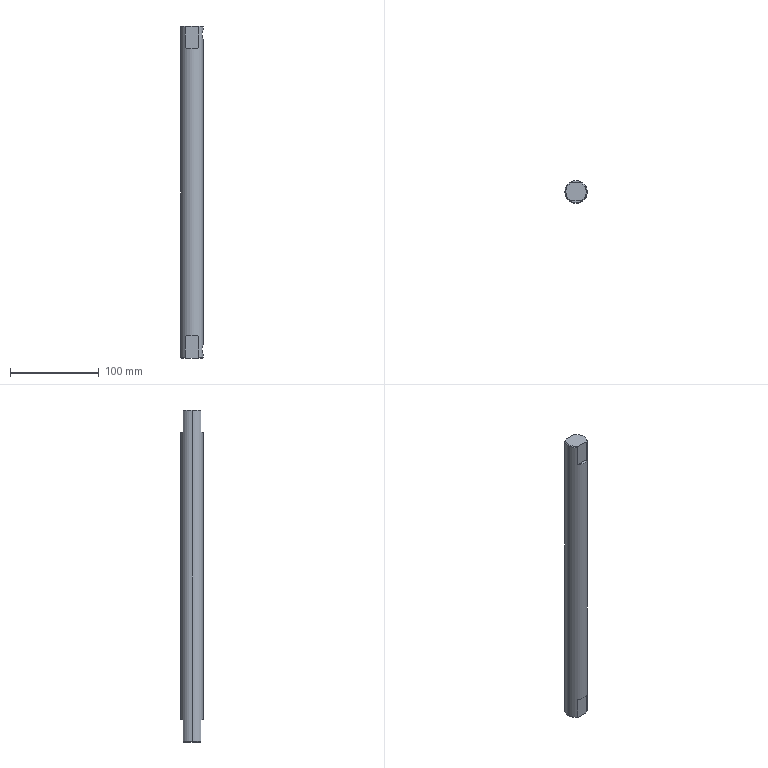Part | SolidWorks | features ICE 2, Chamfer 1, Extrusion 1, MirrorPattern 1 | 1 solid | 24 faces | box 25 x 25 x 374 mm | volume 180094 mm3 | plane 12 | cylinder 6 | cone 6 | commonest cylinder face diameters 11 x4 25 x2
STEP:
#1=CARTESIAN_POINT('',(7.5,0.,-172.));
#2=VERTEX_POINT('',#1);
#3=CARTESIAN_POINT('',(7.5,0.,-183.));
#4=VERTEX_POINT('',#3);
#5=CARTESIAN_POINT('',(7.5,0.,-177.5));
#6=DIRECTION('',(1.,0.,0.));
#7=DIRECTION('',(0.,0.,1.));
#8=AXIS2_PLACEMENT_3D('',#5,#6,#7);
#9=CIRCLE('',#8,5.5);
#10=EDGE_CURVE('',#2,#4,#9,.T.);
#11=ORIENTED_EDGE('',*,*,#10,.F.);
#12=CARTESIAN_POINT('',(12.5,0.,-172.));
#13=VERTEX_POINT('',#12);
#14=CARTESIAN_POINT('',(7.5,0.,-172.));
#15=DIRECTION('',(1.,0.,0.));
#16=VECTOR('',#15,1000.);
#17=LINE('',#14,#16);
#18=EDGE_CURVE('',#2,#13,#17,.T.);
#19=ORIENTED_EDGE('',*,*,#18,.T.);
#20=CARTESIAN_POINT('',(12.5,0.,-183.));
#21=VERTEX_POINT('',#20);
#22=CARTESIAN_POINT('',(12.5,0.,-183.));
#23=CARTESIAN_POINT('',(12.5,-0.3685,-183.));
#24=CARTESIAN_POINT('',(12.484,-0.73,-182.963));
#25=CARTESIAN_POINT('',(12.422,-1.44,-182.821));
#26=CARTESIAN_POINT('',(12.376,-1.792,-182.712));
#27=CARTESIAN_POINT('',(12.261,-2.456,-182.434));
#28=CARTESIAN_POINT('',(12.193,-2.77,-182.265));
#29=CARTESIAN_POINT('',(12.08,-3.216,-181.965));
#30=CARTESIAN_POINT('',(12.041,-3.361,-181.857));
#31=CARTESIAN_POINT('',(11.96,-3.636,-181.631));
#32=CARTESIAN_POINT('',(11.92,-3.767,-181.511));
#33=CARTESIAN_POINT('',(11.797,-4.142,-181.135));
#34=CARTESIAN_POINT('',(11.713,-4.369,-180.86));
#35=CARTESIAN_POINT('',(11.557,-4.768,-180.264));
#36=CARTESIAN_POINT('',(11.485,-4.937,-179.951));
#37=CARTESIAN_POINT('',(11.393,-5.144,-179.456));
#38=CARTESIAN_POINT('',(11.365,-5.205,-179.287));
#39=CARTESIAN_POINT('',(11.316,-5.311,-178.94));
#40=CARTESIAN_POINT('',(11.294,-5.356,-178.762));
#41=CARTESIAN_POINT('',(11.243,-5.464,-178.228));
#42=CARTESIAN_POINT('',(11.225,-5.5,-177.868));
#43=CARTESIAN_POINT('',(11.225,-5.5,-177.322));
#44=CARTESIAN_POINT('',(11.229,-5.491,-177.138));
#45=CARTESIAN_POINT('',(11.247,-5.455,-176.773));
#46=CARTESIAN_POINT('',(11.26,-5.428,-176.593));
#47=CARTESIAN_POINT('',(11.311,-5.321,-176.06));
#48=CARTESIAN_POINT('',(11.362,-5.214,-175.713));
#49=CARTESIAN_POINT('',(11.486,-4.935,-175.045));
#50=CARTESIAN_POINT('',(11.558,-4.765,-174.731));
#51=CARTESIAN_POINT('',(11.714,-4.369,-174.14));
#52=CARTESIAN_POINT('',(11.798,-4.139,-173.861));
#53=CARTESIAN_POINT('',(11.962,-3.637,-173.359));
#54=CARTESIAN_POINT('',(12.043,-3.364,-173.134));
#55=CARTESIAN_POINT('',(12.156,-2.918,-172.834));
#56=CARTESIAN_POINT('',(12.192,-2.763,-172.741));
#57=CARTESIAN_POINT('',(12.259,-2.446,-172.571));
#58=CARTESIAN_POINT('',(12.291,-2.285,-172.494));
#59=CARTESIAN_POINT('',(12.376,-1.789,-172.287));
#60=CARTESIAN_POINT('',(12.422,-1.445,-172.18));
#61=CARTESIAN_POINT('',(12.484,-0.7246,-172.036));
#62=CARTESIAN_POINT('',(12.5,-0.3631,-172.));
#63=CARTESIAN_POINT('',(12.5,0.,-172.));
#64=B_SPLINE_CURVE_WITH_KNOTS('',3,(#22,#23,#24,#25,#26,#27,#28,#29,#30,#31,#32,#33,#34,#35,#36,#37,#38,#39,#40,#41,#42,#43,#44,#45,#46,#47,#48,#49,#50,#51,#52,#53,#54,#55,#56,#57,#58,#59,#60,#61,#62,#63),.UNSPECIFIED.,.F.,.F.,(4,2,2,2,2,2,2,2,2,2,2,2,2,2,2,2,2,2,2,2,4),(0.,0.001089,0.002178,0.003267,0.003811,0.004355,0.005444,0.006533,0.007078,0.007622,0.008711,0.009255,0.0098,0.01089,0.01198,0.01307,0.01416,0.0147,0.01524,0.01633,0.01742),.UNSPECIFIED.);
#65=EDGE_CURVE('',#21,#13,#64,.T.);
#66=ORIENTED_EDGE('',*,*,#65,.F.);
#67=CARTESIAN_POINT('',(7.5,0.,-183.));
#68=DIRECTION('',(1.,0.,0.));
#69=VECTOR('',#68,1000.);
#70=LINE('',#67,#69);
#71=EDGE_CURVE('',#4,#21,#70,.T.);
#72=ORIENTED_EDGE('',*,*,#71,.F.);
#73=EDGE_LOOP('',(#11,#19,#66,#72));
#74=FACE_OUTER_BOUND('',#73,.T.);
#75=CARTESIAN_POINT('',(7.5,0.,-177.5));
#76=DIRECTION('',(1.,0.,0.));
#77=DIRECTION('',(0.,0.,-1.));
#78=AXIS2_PLACEMENT_3D('',#75,#76,#77);
#79=CYLINDRICAL_SURFACE('',#78,5.5);
#80=ADVANCED_FACE('',(#74),#79,.F.);
#81=CARTESIAN_POINT('',(7.5,0.,183.));
#82=VERTEX_POINT('',#81);
#83=CARTESIAN_POINT('',(7.5,0.,172.));
#84=VERTEX_POINT('',#83);
#85=CARTESIAN_POINT('',(7.5,0.,177.5));
#86=DIRECTION('',(1.,0.,0.));
#87=DIRECTION('',(0.,0.,-1.));
#88=AXIS2_PLACEMENT_3D('',#85,#86,#87);
#89=CIRCLE('',#88,5.5);
#90=EDGE_CURVE('',#82,#84,#89,.T.);
#91=ORIENTED_EDGE('',*,*,#90,.F.);
#92=CARTESIAN_POINT('',(12.5,0.,183.));
#93=VERTEX_POINT('',#92);
#94=CARTESIAN_POINT('',(7.5,0.,183.));
#95=DIRECTION('',(1.,0.,0.));
#96=VECTOR('',#95,1000.);
#97=LINE('',#94,#96);
#98=EDGE_CURVE('',#82,#93,#97,.T.);
#99=ORIENTED_EDGE('',*,*,#98,.T.);
#100=CARTESIAN_POINT('',(12.5,0.,172.));
#101=VERTEX_POINT('',#100);
#102=CARTESIAN_POINT('',(12.5,0.,172.));
#103=CARTESIAN_POINT('',(12.5,-0.3685,172.));
#104=CARTESIAN_POINT('',(12.484,-0.73,172.037));
#105=CARTESIAN_POINT('',(12.422,-1.44,172.179));
#106=CARTESIAN_POINT('',(12.376,-1.792,172.288));
#107=CARTESIAN_POINT('',(12.261,-2.456,172.566));
#108=CARTESIAN_POINT('',(12.193,-2.77,172.735));
#109=CARTESIAN_POINT('',(12.08,-3.216,173.035));
#110=CARTESIAN_POINT('',(12.041,-3.361,173.143));
#111=CARTESIAN_POINT('',(11.96,-3.636,173.369));
#112=CARTESIAN_POINT('',(11.92,-3.767,173.489));
#113=CARTESIAN_POINT('',(11.797,-4.142,173.865));
#114=CARTESIAN_POINT('',(11.713,-4.369,174.14));
#115=CARTESIAN_POINT('',(11.557,-4.768,174.736));
#116=CARTESIAN_POINT('',(11.485,-4.937,175.049));
#117=CARTESIAN_POINT('',(11.393,-5.144,175.544));
#118=CARTESIAN_POINT('',(11.365,-5.205,175.713));
#119=CARTESIAN_POINT('',(11.316,-5.311,176.06));
#120=CARTESIAN_POINT('',(11.294,-5.356,176.238));
#121=CARTESIAN_POINT('',(11.243,-5.464,176.772));
#122=CARTESIAN_POINT('',(11.225,-5.5,177.132));
#123=CARTESIAN_POINT('',(11.225,-5.5,177.678));
#124=CARTESIAN_POINT('',(11.229,-5.491,177.862));
#125=CARTESIAN_POINT('',(11.247,-5.455,178.227));
#126=CARTESIAN_POINT('',(11.26,-5.428,178.407));
#127=CARTESIAN_POINT('',(11.311,-5.321,178.94));
#128=CARTESIAN_POINT('',(11.362,-5.214,179.287));
#129=CARTESIAN_POINT('',(11.486,-4.935,179.955));
#130=CARTESIAN_POINT('',(11.558,-4.765,180.269));
#131=CARTESIAN_POINT('',(11.714,-4.369,180.86));
#132=CARTESIAN_POINT('',(11.798,-4.139,181.139));
#133=CARTESIAN_POINT('',(11.962,-3.637,181.641));
#134=CARTESIAN_POINT('',(12.043,-3.364,181.866));
#135=CARTESIAN_POINT('',(12.156,-2.918,182.166));
#136=CARTESIAN_POINT('',(12.192,-2.763,182.259));
#137=CARTESIAN_POINT('',(12.259,-2.446,182.429));
#138=CARTESIAN_POINT('',(12.291,-2.285,182.506));
#139=CARTESIAN_POINT('',(12.376,-1.789,182.713));
#140=CARTESIAN_POINT('',(12.422,-1.445,182.82));
#141=CARTESIAN_POINT('',(12.484,-0.7246,182.964));
#142=CARTESIAN_POINT('',(12.5,-0.3631,183.));
#143=CARTESIAN_POINT('',(12.5,0.,183.));
#144=B_SPLINE_CURVE_WITH_KNOTS('',3,(#102,#103,#104,#105,#106,#107,#108,#109,#110,#111,#112,#113,#114,#115,#116,#117,#118,#119,#120,#121,#122,#123,#124,#125,#126,#127,#128,#129,#130,#131,#132,#133,#134,#135,#136,#137,#138,#139,#140,#141,#142,#143),.UNSPECIFIED.,.F.,.F.,(4,2,2,2,2,2,2,2,2,2,2,2,2,2,2,2,2,2,2,2,4),(0.,0.001089,0.002178,0.003267,0.003811,0.004355,0.005444,0.006533,0.007078,0.007622,0.008711,0.009255,0.0098,0.01089,0.01198,0.01307,0.01416,0.0147,0.01524,0.01633,0.01742),.UNSPECIFIED.);
#145=EDGE_CURVE('',#101,#93,#144,.T.);
#146=ORIENTED_EDGE('',*,*,#145,.F.);
#147=CARTESIAN_POINT('',(7.5,0.,172.));
#148=DIRECTION('',(1.,0.,0.));
#149=VECTOR('',#148,1000.);
#150=LINE('',#147,#149);
#151=EDGE_CURVE('',#84,#101,#150,.T.);
#152=ORIENTED_EDGE('',*,*,#151,.F.);
#153=EDGE_LOOP('',(#91,#99,#146,#152));
#154=FACE_OUTER_BOUND('',#153,.T.);
#155=CARTESIAN_POINT('',(7.5,0.,177.5));
#156=DIRECTION('',(1.,0.,0.));
#157=DIRECTION('',(0.,0.,-1.));
#158=AXIS2_PLACEMENT_3D('',#155,#156,#157);
#159=CYLINDRICAL_SURFACE('',#158,5.5);
#160=ADVANCED_FACE('',(#154),#159,.F.);
#161=CARTESIAN_POINT('',(-11.5,0.,187.));
#162=VERTEX_POINT('',#161);
#163=CARTESIAN_POINT('',(-5.679,-10.,187.));
#164=VERTEX_POINT('',#163);
#165=CARTESIAN_POINT('',(0.,0.,187.));
#166=DIRECTION('',(0.,0.,1.));
#167=DIRECTION('',(1.,0.,0.));
#168=AXIS2_PLACEMENT_3D('',#165,#166,#167);
#169=CIRCLE('',#168,11.5);
#170=EDGE_CURVE('',#162,#164,#169,.T.);
#171=ORIENTED_EDGE('',*,*,#170,.F.);
#172=CARTESIAN_POINT('',(-12.5,0.,186.));
#173=VERTEX_POINT('',#172);
#174=CARTESIAN_POINT('',(-11.5,0.,187.));
#175=DIRECTION('',(-0.7071,0.,-0.7071));
#176=VECTOR('',#175,1000.);
#177=LINE('',#174,#176);
#178=EDGE_CURVE('',#162,#173,#177,.T.);
#179=ORIENTED_EDGE('',*,*,#178,.T.);
#180=CARTESIAN_POINT('',(-7.5,-10.,186.));
#181=VERTEX_POINT('',#180);
#182=CARTESIAN_POINT('',(0.,0.,186.));
#183=DIRECTION('',(0.,0.,-1.));
#184=DIRECTION('',(1.,0.,0.));
#185=AXIS2_PLACEMENT_3D('',#182,#183,#184);
#186=CIRCLE('',#185,12.5);
#187=EDGE_CURVE('',#181,#173,#186,.T.);
#188=ORIENTED_EDGE('',*,*,#187,.F.);
#189=CARTESIAN_POINT('',(-5.679,-10.,187.));
#190=CARTESIAN_POINT('',(-6.301,-10.,186.693));
#191=CARTESIAN_POINT('',(-6.906,-10.,186.356));
#192=CARTESIAN_POINT('',(-7.5,-10.,186.));
#193=B_SPLINE_CURVE_WITH_KNOTS('',3,(#189,#190,#191,#192),.UNSPECIFIED.,.F.,.F.,(4,4),(0.03752,0.03962),.UNSPECIFIED.);
#194=EDGE_CURVE('',#164,#181,#193,.T.);
#195=ORIENTED_EDGE('',*,*,#194,.F.);
#196=EDGE_LOOP('',(#171,#179,#188,#195));
#197=FACE_OUTER_BOUND('',#196,.T.);
#198=CARTESIAN_POINT('',(0.,0.,187.));
#199=DIRECTION('',(0.,0.,-1.));
#200=DIRECTION('',(-1.,0.,0.));
#201=AXIS2_PLACEMENT_3D('',#198,#199,#200);
#202=CONICAL_SURFACE('',#201,11.5,0.7854);
#203=ADVANCED_FACE('',(#197),#202,.T.);
#204=CARTESIAN_POINT('',(11.5,0.,-187.));
#205=VERTEX_POINT('',#204);
#206=CARTESIAN_POINT('',(5.679,-10.,-187.));
#207=VERTEX_POINT('',#206);
#208=CARTESIAN_POINT('',(0.,0.,-187.));
#209=DIRECTION('',(0.,0.,-1.));
#210=DIRECTION('',(1.,0.,0.));
#211=AXIS2_PLACEMENT_3D('',#208,#209,#210);
#212=CIRCLE('',#211,11.5);
#213=EDGE_CURVE('',#205,#207,#212,.T.);
#214=ORIENTED_EDGE('',*,*,#213,.F.);
#215=CARTESIAN_POINT('',(12.5,0.,-186.));
#216=VERTEX_POINT('',#215);
#217=CARTESIAN_POINT('',(12.5,0.,-186.));
#218=DIRECTION('',(0.7071,0.,0.7071));
#219=VECTOR('',#218,1000.);
#220=LINE('',#217,#219);
#221=EDGE_CURVE('',#205,#216,#220,.T.);
#222=ORIENTED_EDGE('',*,*,#221,.T.);
#223=CARTESIAN_POINT('',(7.5,-10.,-186.));
#224=VERTEX_POINT('',#223);
#225=CARTESIAN_POINT('',(0.,0.,-186.));
#226=DIRECTION('',(0.,0.,1.));
#227=DIRECTION('',(1.,0.,0.));
#228=AXIS2_PLACEMENT_3D('',#225,#226,#227);
#229=CIRCLE('',#228,12.5);
#230=EDGE_CURVE('',#224,#216,#229,.T.);
#231=ORIENTED_EDGE('',*,*,#230,.F.);
#232=CARTESIAN_POINT('',(7.5,-10.,-186.));
#233=CARTESIAN_POINT('',(6.905,-10.,-186.357));
#234=CARTESIAN_POINT('',(6.299,-10.,-186.694));
#235=CARTESIAN_POINT('',(5.679,-10.,-187.));
#236=B_SPLINE_CURVE_WITH_KNOTS('',3,(#232,#233,#234,#235),.UNSPECIFIED.,.F.,.F.,(4,4),(0.02358,0.02565),.UNSPECIFIED.);
#237=EDGE_CURVE('',#224,#207,#236,.T.);
#238=ORIENTED_EDGE('',*,*,#237,.T.);
#239=EDGE_LOOP('',(#214,#222,#231,#238));
#240=FACE_OUTER_BOUND('',#239,.T.);
#241=CARTESIAN_POINT('',(0.,0.,-186.));
#242=DIRECTION('',(0.,0.,1.));
#243=DIRECTION('',(1.,0.,0.));
#244=AXIS2_PLACEMENT_3D('',#241,#242,#243);
#245=CONICAL_SURFACE('',#244,12.5,0.7854);
#246=ADVANCED_FACE('',(#240),#245,.T.);
#247=CARTESIAN_POINT('',(7.5,10.,186.));
#248=VERTEX_POINT('',#247);
#249=CARTESIAN_POINT('',(12.5,0.,186.));
#250=VERTEX_POINT('',#249);
#251=CARTESIAN_POINT('',(0.,0.,186.));
#252=DIRECTION('',(0.,0.,-1.));
#253=DIRECTION('',(1.,0.,0.));
#254=AXIS2_PLACEMENT_3D('',#251,#252,#253);
#255=CIRCLE('',#254,12.5);
#256=EDGE_CURVE('',#248,#250,#255,.T.);
#257=ORIENTED_EDGE('',*,*,#256,.T.);
#258=CARTESIAN_POINT('',(12.5,0.,187.));
#259=DIRECTION('',(0.,0.,-1.));
#260=VECTOR('',#259,1000.);
#261=LINE('',#258,#260);
#262=EDGE_CURVE('',#250,#93,#261,.T.);
#263=ORIENTED_EDGE('',*,*,#262,.T.);
#264=CARTESIAN_POINT('',(12.5,0.,183.));
#265=CARTESIAN_POINT('',(12.5,0.1813,183.));
#266=CARTESIAN_POINT('',(12.496,0.3631,182.991));
#267=CARTESIAN_POINT('',(12.48,0.7273,182.955));
#268=CARTESIAN_POINT('',(12.468,0.9095,182.927));
#269=CARTESIAN_POINT('',(12.421,1.444,182.82));
#270=CARTESIAN_POINT('',(12.376,1.788,182.714));
#271=CARTESIAN_POINT('',(12.29,2.289,182.505));
#272=CARTESIAN_POINT('',(12.258,2.453,182.426));
#273=CARTESIAN_POINT('',(12.191,2.769,182.256));
#274=CARTESIAN_POINT('',(12.155,2.921,182.163));
#275=CARTESIAN_POINT('',(12.043,3.364,181.866));
#276=CARTESIAN_POINT('',(11.961,3.641,181.637));
#277=CARTESIAN_POINT('',(11.796,4.145,181.133));
#278=CARTESIAN_POINT('',(11.713,4.369,180.859));
#279=CARTESIAN_POINT('',(11.558,4.765,180.27));
#280=CARTESIAN_POINT('',(11.484,4.938,179.949));
#281=CARTESIAN_POINT('',(11.362,5.214,179.288));
#282=CARTESIAN_POINT('',(11.312,5.319,178.945));
#283=CARTESIAN_POINT('',(11.261,5.427,178.412));
#284=CARTESIAN_POINT('',(11.247,5.454,178.229));
#285=CARTESIAN_POINT('',(11.229,5.491,177.866));
#286=CARTESIAN_POINT('',(11.225,5.5,177.684));
#287=CARTESIAN_POINT('',(11.225,5.5,177.14));
#288=CARTESIAN_POINT('',(11.243,5.465,176.777));
#289=CARTESIAN_POINT('',(11.311,5.32,176.059));
#290=CARTESIAN_POINT('',(11.361,5.214,175.714));
#291=CARTESIAN_POINT('',(11.484,4.938,175.051));
#292=CARTESIAN_POINT('',(11.558,4.766,174.731));
#293=CARTESIAN_POINT('',(11.713,4.369,174.14));
#294=CARTESIAN_POINT('',(11.796,4.144,173.866));
#295=CARTESIAN_POINT('',(11.962,3.639,173.36));
#296=CARTESIAN_POINT('',(12.043,3.363,173.134));
#297=CARTESIAN_POINT('',(12.155,2.921,172.837));
#298=CARTESIAN_POINT('',(12.191,2.769,172.744));
#299=CARTESIAN_POINT('',(12.258,2.454,172.574));
#300=CARTESIAN_POINT('',(12.29,2.29,172.496));
#301=CARTESIAN_POINT('',(12.376,1.789,172.286));
#302=CARTESIAN_POINT('',(12.421,1.445,172.181));
#303=CARTESIAN_POINT('',(12.483,0.7361,172.038));
#304=CARTESIAN_POINT('',(12.5,0.3681,172.));
#305=CARTESIAN_POINT('',(12.5,0.,172.));
#306=B_SPLINE_CURVE_WITH_KNOTS('',3,(#264,#265,#266,#267,#268,#269,#270,#271,#272,#273,#274,#275,#276,#277,#278,#279,#280,#281,#282,#283,#284,#285,#286,#287,#288,#289,#290,#291,#292,#293,#294,#295,#296,#297,#298,#299,#300,#301,#302,#303,#304,#305),.UNSPECIFIED.,.F.,.F.,(4,2,2,2,2,2,2,2,2,2,2,2,2,2,2,2,2,2,2,2,4),(0.01742,0.01797,0.01851,0.0196,0.02014,0.02068,0.02177,0.02286,0.02395,0.02504,0.02558,0.02612,0.02721,0.0283,0.02939,0.03047,0.03156,0.03211,0.03265,0.03374,0.03483),.UNSPECIFIED.);
#307=EDGE_CURVE('',#93,#101,#306,.T.);
#308=ORIENTED_EDGE('',*,*,#307,.T.);
#309=CARTESIAN_POINT('',(12.5,0.,187.));
#310=DIRECTION('',(0.,0.,-1.));
#311=VECTOR('',#310,1000.);
#312=LINE('',#309,#311);
#313=EDGE_CURVE('',#101,#13,#312,.T.);
#314=ORIENTED_EDGE('',*,*,#313,.T.);
#315=CARTESIAN_POINT('',(12.5,0.,-172.));
#316=CARTESIAN_POINT('',(12.5,0.1813,-172.));
#317=CARTESIAN_POINT('',(12.496,0.3631,-172.009));
#318=CARTESIAN_POINT('',(12.48,0.7273,-172.045));
#319=CARTESIAN_POINT('',(12.468,0.9095,-172.073));
#320=CARTESIAN_POINT('',(12.421,1.444,-172.18));
#321=CARTESIAN_POINT('',(12.376,1.788,-172.286));
#322=CARTESIAN_POINT('',(12.29,2.289,-172.495));
#323=CARTESIAN_POINT('',(12.258,2.453,-172.574));
#324=CARTESIAN_POINT('',(12.191,2.769,-172.744));
#325=CARTESIAN_POINT('',(12.155,2.921,-172.837));
#326=CARTESIAN_POINT('',(12.043,3.364,-173.134));
#327=CARTESIAN_POINT('',(11.961,3.641,-173.363));
#328=CARTESIAN_POINT('',(11.796,4.145,-173.867));
#329=CARTESIAN_POINT('',(11.713,4.369,-174.141));
#330=CARTESIAN_POINT('',(11.558,4.765,-174.73));
#331=CARTESIAN_POINT('',(11.484,4.938,-175.051));
#332=CARTESIAN_POINT('',(11.362,5.214,-175.712));
#333=CARTESIAN_POINT('',(11.312,5.319,-176.055));
#334=CARTESIAN_POINT('',(11.261,5.427,-176.588));
#335=CARTESIAN_POINT('',(11.247,5.454,-176.771));
#336=CARTESIAN_POINT('',(11.229,5.491,-177.134));
#337=CARTESIAN_POINT('',(11.225,5.5,-177.316));
#338=CARTESIAN_POINT('',(11.225,5.5,-177.86));
#339=CARTESIAN_POINT('',(11.243,5.465,-178.223));
#340=CARTESIAN_POINT('',(11.311,5.32,-178.941));
#341=CARTESIAN_POINT('',(11.361,5.214,-179.286));
#342=CARTESIAN_POINT('',(11.484,4.938,-179.949));
#343=CARTESIAN_POINT('',(11.558,4.766,-180.269));
#344=CARTESIAN_POINT('',(11.713,4.369,-180.86));
#345=CARTESIAN_POINT('',(11.796,4.144,-181.134));
#346=CARTESIAN_POINT('',(11.962,3.639,-181.64));
#347=CARTESIAN_POINT('',(12.043,3.363,-181.866));
#348=CARTESIAN_POINT('',(12.155,2.921,-182.163));
#349=CARTESIAN_POINT('',(12.191,2.769,-182.256));
#350=CARTESIAN_POINT('',(12.258,2.454,-182.426));
#351=CARTESIAN_POINT('',(12.29,2.29,-182.504));
#352=CARTESIAN_POINT('',(12.376,1.789,-182.714));
#353=CARTESIAN_POINT('',(12.421,1.445,-182.819));
#354=CARTESIAN_POINT('',(12.483,0.7361,-182.962));
#355=CARTESIAN_POINT('',(12.5,0.3681,-183.));
#356=CARTESIAN_POINT('',(12.5,0.,-183.));
#357=B_SPLINE_CURVE_WITH_KNOTS('',3,(#315,#316,#317,#318,#319,#320,#321,#322,#323,#324,#325,#326,#327,#328,#329,#330,#331,#332,#333,#334,#335,#336,#337,#338,#339,#340,#341,#342,#343,#344,#345,#346,#347,#348,#349,#350,#351,#352,#353,#354,#355,#356),.UNSPECIFIED.,.F.,.F.,(4,2,2,2,2,2,2,2,2,2,2,2,2,2,2,2,2,2,2,2,4),(0.01742,0.01797,0.01851,0.0196,0.02014,0.02068,0.02177,0.02286,0.02395,0.02504,0.02558,0.02612,0.02721,0.0283,0.02939,0.03047,0.03156,0.03211,0.03265,0.03374,0.03483),.UNSPECIFIED.);
#358=EDGE_CURVE('',#13,#21,#357,.T.);
#359=ORIENTED_EDGE('',*,*,#358,.T.);
#360=CARTESIAN_POINT('',(12.5,0.,187.));
#361=DIRECTION('',(0.,0.,-1.));
#362=VECTOR('',#361,1000.);
#363=LINE('',#360,#362);
#364=EDGE_CURVE('',#21,#216,#363,.T.);
#365=ORIENTED_EDGE('',*,*,#364,.T.);
#366=CARTESIAN_POINT('',(7.5,10.,-186.));
#367=VERTEX_POINT('',#366);
#368=CARTESIAN_POINT('',(0.,0.,-186.));
#369=DIRECTION('',(0.,0.,1.));
#370=DIRECTION('',(1.,0.,0.));
#371=AXIS2_PLACEMENT_3D('',#368,#369,#370);
#372=CIRCLE('',#371,12.5);
#373=EDGE_CURVE('',#216,#367,#372,.T.);
#374=ORIENTED_EDGE('',*,*,#373,.T.);
#375=CARTESIAN_POINT('',(7.5,10.,-162.));
#376=VERTEX_POINT('',#375);
#377=CARTESIAN_POINT('',(7.5,10.,187.));
#378=DIRECTION('',(0.,0.,-1.));
#379=VECTOR('',#378,1000.);
#380=LINE('',#377,#379);
#381=EDGE_CURVE('',#376,#367,#380,.T.);
#382=ORIENTED_EDGE('',*,*,#381,.F.);
#383=CARTESIAN_POINT('',(-7.5,10.,-162.));
#384=VERTEX_POINT('',#383);
#385=CARTESIAN_POINT('',(0.,0.,-162.));
#386=DIRECTION('',(0.,0.,1.));
#387=DIRECTION('',(1.,0.,0.));
#388=AXIS2_PLACEMENT_3D('',#385,#386,#387);
#389=CIRCLE('',#388,12.5);
#390=EDGE_CURVE('',#376,#384,#389,.T.);
#391=ORIENTED_EDGE('',*,*,#390,.T.);
#392=CARTESIAN_POINT('',(-7.5,10.,-186.));
#393=VERTEX_POINT('',#392);
#394=CARTESIAN_POINT('',(-7.5,10.,187.));
#395=DIRECTION('',(0.,0.,1.));
#396=VECTOR('',#395,1000.);
#397=LINE('',#394,#396);
#398=EDGE_CURVE('',#393,#384,#397,.T.);
#399=ORIENTED_EDGE('',*,*,#398,.F.);
#400=CARTESIAN_POINT('',(-12.5,0.,-186.));
#401=VERTEX_POINT('',#400);
#402=CARTESIAN_POINT('',(0.,0.,-186.));
#403=DIRECTION('',(0.,0.,1.));
#404=DIRECTION('',(1.,0.,0.));
#405=AXIS2_PLACEMENT_3D('',#402,#403,#404);
#406=CIRCLE('',#405,12.5);
#407=EDGE_CURVE('',#393,#401,#406,.T.);
#408=ORIENTED_EDGE('',*,*,#407,.T.);
#409=CARTESIAN_POINT('',(-12.5,0.,187.));
#410=DIRECTION('',(0.,0.,-1.));
#411=VECTOR('',#410,1000.);
#412=LINE('',#409,#411);
#413=EDGE_CURVE('',#173,#401,#412,.T.);
#414=ORIENTED_EDGE('',*,*,#413,.F.);
#415=CARTESIAN_POINT('',(-7.5,10.,186.));
#416=VERTEX_POINT('',#415);
#417=CARTESIAN_POINT('',(0.,0.,186.));
#418=DIRECTION('',(0.,0.,-1.));
#419=DIRECTION('',(1.,0.,0.));
#420=AXIS2_PLACEMENT_3D('',#417,#418,#419);
#421=CIRCLE('',#420,12.5);
#422=EDGE_CURVE('',#173,#416,#421,.T.);
#423=ORIENTED_EDGE('',*,*,#422,.T.);
#424=CARTESIAN_POINT('',(-7.5,10.,162.));
#425=VERTEX_POINT('',#424);
#426=CARTESIAN_POINT('',(-7.5,10.,187.));
#427=DIRECTION('',(0.,0.,-1.));
#428=VECTOR('',#427,1000.);
#429=LINE('',#426,#428);
#430=EDGE_CURVE('',#416,#425,#429,.T.);
#431=ORIENTED_EDGE('',*,*,#430,.T.);
#432=CARTESIAN_POINT('',(7.5,10.,162.));
#433=VERTEX_POINT('',#432);
#434=CARTESIAN_POINT('',(0.,0.,162.));
#435=DIRECTION('',(0.,0.,-1.));
#436=DIRECTION('',(-1.,0.,0.));
#437=AXIS2_PLACEMENT_3D('',#434,#435,#436);
#438=CIRCLE('',#437,12.5);
#439=EDGE_CURVE('',#425,#433,#438,.T.);
#440=ORIENTED_EDGE('',*,*,#439,.T.);
#441=CARTESIAN_POINT('',(7.5,10.,187.));
#442=DIRECTION('',(0.,0.,1.));
#443=VECTOR('',#442,1000.);
#444=LINE('',#441,#443);
#445=EDGE_CURVE('',#433,#248,#444,.T.);
#446=ORIENTED_EDGE('',*,*,#445,.T.);
#447=EDGE_LOOP('',(#257,#263,#308,#314,#359,#365,#374,#382,#391,#399,#408,#414,#423,#431,#440,#446));
#448=FACE_OUTER_BOUND('',#447,.T.);
#449=CARTESIAN_POINT('',(0.,0.,187.));
#450=DIRECTION('',(0.,0.,-1.));
#451=DIRECTION('',(-1.,0.,0.));
#452=AXIS2_PLACEMENT_3D('',#449,#450,#451);
#453=CYLINDRICAL_SURFACE('',#452,12.5);
#454=ADVANCED_FACE('',(#448),#453,.T.);
#455=ORIENTED_EDGE('',*,*,#262,.F.);
#456=CARTESIAN_POINT('',(7.5,-10.,186.));
#457=VERTEX_POINT('',#456);
#458=CARTESIAN_POINT('',(0.,0.,186.));
#459=DIRECTION('',(0.,0.,-1.));
#460=DIRECTION('',(1.,0.,0.));
#461=AXIS2_PLACEMENT_3D('',#458,#459,#460);
#462=CIRCLE('',#461,12.5);
#463=EDGE_CURVE('',#250,#457,#462,.T.);
#464=ORIENTED_EDGE('',*,*,#463,.T.);
#465=CARTESIAN_POINT('',(7.5,-10.,162.));
#466=VERTEX_POINT('',#465);
#467=CARTESIAN_POINT('',(7.5,-10.,187.));
#468=DIRECTION('',(0.,0.,-1.));
#469=VECTOR('',#468,1000.);
#470=LINE('',#467,#469);
#471=EDGE_CURVE('',#457,#466,#470,.T.);
#472=ORIENTED_EDGE('',*,*,#471,.T.);
#473=CARTESIAN_POINT('',(-7.5,-10.,162.));
#474=VERTEX_POINT('',#473);
#475=CARTESIAN_POINT('',(0.,0.,162.));
#476=DIRECTION('',(0.,0.,1.));
#477=DIRECTION('',(1.,0.,0.));
#478=AXIS2_PLACEMENT_3D('',#475,#476,#477);
#479=CIRCLE('',#478,12.5);
#480=EDGE_CURVE('',#474,#466,#479,.T.);
#481=ORIENTED_EDGE('',*,*,#480,.F.);
#482=CARTESIAN_POINT('',(-7.5,-10.,187.));
#483=DIRECTION('',(0.,0.,1.));
#484=VECTOR('',#483,1000.);
#485=LINE('',#482,#484);
#486=EDGE_CURVE('',#474,#181,#485,.T.);
#487=ORIENTED_EDGE('',*,*,#486,.T.);
#488=ORIENTED_EDGE('',*,*,#187,.T.);
#489=ORIENTED_EDGE('',*,*,#413,.T.);
#490=CARTESIAN_POINT('',(-7.5,-10.,-186.));
#491=VERTEX_POINT('',#490);
#492=CARTESIAN_POINT('',(0.,0.,-186.));
#493=DIRECTION('',(0.,0.,1.));
#494=DIRECTION('',(1.,0.,0.));
#495=AXIS2_PLACEMENT_3D('',#492,#493,#494);
#496=CIRCLE('',#495,12.5);
#497=EDGE_CURVE('',#401,#491,#496,.T.);
#498=ORIENTED_EDGE('',*,*,#497,.T.);
#499=CARTESIAN_POINT('',(-7.5,-10.,-162.));
#500=VERTEX_POINT('',#499);
#501=CARTESIAN_POINT('',(-7.5,-10.,187.));
#502=DIRECTION('',(0.,0.,-1.));
#503=VECTOR('',#502,1000.);
#504=LINE('',#501,#503);
#505=EDGE_CURVE('',#500,#491,#504,.T.);
#506=ORIENTED_EDGE('',*,*,#505,.F.);
#507=CARTESIAN_POINT('',(7.5,-10.,-162.));
#508=VERTEX_POINT('',#507);
#509=CARTESIAN_POINT('',(0.,0.,-162.));
#510=DIRECTION('',(0.,0.,-1.));
#511=DIRECTION('',(-1.,0.,0.));
#512=AXIS2_PLACEMENT_3D('',#509,#510,#511);
#513=CIRCLE('',#512,12.5);
#514=EDGE_CURVE('',#508,#500,#513,.T.);
#515=ORIENTED_EDGE('',*,*,#514,.F.);
#516=CARTESIAN_POINT('',(7.5,-10.,187.));
#517=DIRECTION('',(0.,0.,1.));
#518=VECTOR('',#517,1000.);
#519=LINE('',#516,#518);
#520=EDGE_CURVE('',#224,#508,#519,.T.);
#521=ORIENTED_EDGE('',*,*,#520,.F.);
#522=ORIENTED_EDGE('',*,*,#230,.T.);
#523=ORIENTED_EDGE('',*,*,#364,.F.);
#524=ORIENTED_EDGE('',*,*,#65,.T.);
#525=ORIENTED_EDGE('',*,*,#313,.F.);
#526=ORIENTED_EDGE('',*,*,#145,.T.);
#527=EDGE_LOOP('',(#455,#464,#472,#481,#487,#488,#489,#498,#506,#515,#521,#522,#523,#524,#525,#526));
#528=FACE_OUTER_BOUND('',#527,.T.);
#529=CARTESIAN_POINT('',(0.,0.,187.));
#530=DIRECTION('',(0.,0.,-1.));
#531=DIRECTION('',(-1.,0.,0.));
#532=AXIS2_PLACEMENT_3D('',#529,#530,#531);
#533=CYLINDRICAL_SURFACE('',#532,12.5);
#534=ADVANCED_FACE('',(#528),#533,.T.);
#535=CARTESIAN_POINT('',(-5.679,-10.,-187.));
#536=VERTEX_POINT('',#535);
#537=CARTESIAN_POINT('',(-12.5,-10.,-187.));
#538=DIRECTION('',(-1.,0.,0.));
#539=VECTOR('',#538,1000.);
#540=LINE('',#537,#539);
#541=EDGE_CURVE('',#207,#536,#540,.T.);
#542=ORIENTED_EDGE('',*,*,#541,.T.);
#543=CARTESIAN_POINT('',(-5.679,10.,-187.));
#544=VERTEX_POINT('',#543);
#545=CARTESIAN_POINT('',(0.,0.,-187.));
#546=DIRECTION('',(0.,0.,-1.));
#547=DIRECTION('',(1.,0.,0.));
#548=AXIS2_PLACEMENT_3D('',#545,#546,#547);
#549=CIRCLE('',#548,11.5);
#550=EDGE_CURVE('',#536,#544,#549,.T.);
#551=ORIENTED_EDGE('',*,*,#550,.T.);
#552=CARTESIAN_POINT('',(5.679,10.,-187.));
#553=VERTEX_POINT('',#552);
#554=CARTESIAN_POINT('',(-12.5,10.,-187.));
#555=DIRECTION('',(-1.,0.,0.));
#556=VECTOR('',#555,1000.);
#557=LINE('',#554,#556);
#558=EDGE_CURVE('',#553,#544,#557,.T.);
#559=ORIENTED_EDGE('',*,*,#558,.F.);
#560=CARTESIAN_POINT('',(0.,0.,-187.));
#561=DIRECTION('',(0.,0.,-1.));
#562=DIRECTION('',(1.,0.,0.));
#563=AXIS2_PLACEMENT_3D('',#560,#561,#562);
#564=CIRCLE('',#563,11.5);
#565=EDGE_CURVE('',#553,#205,#564,.T.);
#566=ORIENTED_EDGE('',*,*,#565,.T.);
#567=ORIENTED_EDGE('',*,*,#213,.T.);
#568=EDGE_LOOP('',(#542,#551,#559,#566,#567));
#569=FACE_OUTER_BOUND('',#568,.T.);
#570=CARTESIAN_POINT('',(0.,0.,-187.));
#571=DIRECTION('',(0.,0.,1.));
#572=DIRECTION('',(1.,0.,0.));
#573=AXIS2_PLACEMENT_3D('',#570,#571,#572);
#574=PLANE('',#573);
#575=ADVANCED_FACE('',(#569),#574,.F.);
#576=ORIENTED_EDGE('',*,*,#221,.F.);
#577=ORIENTED_EDGE('',*,*,#565,.F.);
#578=CARTESIAN_POINT('',(5.679,10.,-187.));
#579=CARTESIAN_POINT('',(6.301,10.,-186.693));
#580=CARTESIAN_POINT('',(6.906,10.,-186.356));
#581=CARTESIAN_POINT('',(7.5,10.,-186.));
#582=B_SPLINE_CURVE_WITH_KNOTS('',3,(#578,#579,#580,#581),.UNSPECIFIED.,.F.,.F.,(4,4),(0.03752,0.03962),.UNSPECIFIED.);
#583=EDGE_CURVE('',#553,#367,#582,.T.);
#584=ORIENTED_EDGE('',*,*,#583,.T.);
#585=ORIENTED_EDGE('',*,*,#373,.F.);
#586=EDGE_LOOP('',(#576,#577,#584,#585));
#587=FACE_OUTER_BOUND('',#586,.T.);
#588=CARTESIAN_POINT('',(0.,0.,-186.));
#589=DIRECTION('',(0.,0.,1.));
#590=DIRECTION('',(1.,0.,0.));
#591=AXIS2_PLACEMENT_3D('',#588,#589,#590);
#592=CONICAL_SURFACE('',#591,12.5,0.7854);
#593=ADVANCED_FACE('',(#587),#592,.T.);
#594=ORIENTED_EDGE('',*,*,#550,.F.);
#595=CARTESIAN_POINT('',(-5.679,-10.,-187.));
#596=CARTESIAN_POINT('',(-6.301,-10.,-186.693));
#597=CARTESIAN_POINT('',(-6.906,-10.,-186.356));
#598=CARTESIAN_POINT('',(-7.5,-10.,-186.));
#599=B_SPLINE_CURVE_WITH_KNOTS('',3,(#595,#596,#597,#598),.UNSPECIFIED.,.F.,.F.,(4,4),(0.03752,0.03962),.UNSPECIFIED.);
#600=EDGE_CURVE('',#536,#491,#599,.T.);
#601=ORIENTED_EDGE('',*,*,#600,.T.);
#602=ORIENTED_EDGE('',*,*,#497,.F.);
#603=ORIENTED_EDGE('',*,*,#407,.F.);
#604=CARTESIAN_POINT('',(-7.5,10.,-186.));
#605=CARTESIAN_POINT('',(-6.905,10.,-186.357));
#606=CARTESIAN_POINT('',(-6.299,10.,-186.694));
#607=CARTESIAN_POINT('',(-5.679,10.,-187.));
#608=B_SPLINE_CURVE_WITH_KNOTS('',3,(#604,#605,#606,#607),.UNSPECIFIED.,.F.,.F.,(4,4),(0.02358,0.02565),.UNSPECIFIED.);
#609=EDGE_CURVE('',#393,#544,#608,.T.);
#610=ORIENTED_EDGE('',*,*,#609,.T.);
#611=EDGE_LOOP('',(#594,#601,#602,#603,#610));
#612=FACE_OUTER_BOUND('',#611,.T.);
#613=CARTESIAN_POINT('',(0.,0.,-186.));
#614=DIRECTION('',(0.,0.,1.));
#615=DIRECTION('',(1.,0.,0.));
#616=AXIS2_PLACEMENT_3D('',#613,#614,#615);
#617=CONICAL_SURFACE('',#616,12.5,0.7854);
#618=ADVANCED_FACE('',(#612),#617,.T.);
#619=CARTESIAN_POINT('',(5.679,-10.,187.));
#620=VERTEX_POINT('',#619);
#621=CARTESIAN_POINT('',(7.5,-10.,186.));
#622=CARTESIAN_POINT('',(6.905,-10.,186.357));
#623=CARTESIAN_POINT('',(6.299,-10.,186.694));
#624=CARTESIAN_POINT('',(5.679,-10.,187.));
#625=B_SPLINE_CURVE_WITH_KNOTS('',3,(#621,#622,#623,#624),.UNSPECIFIED.,.F.,.F.,(4,4),(0.02358,0.02565),.UNSPECIFIED.);
#626=EDGE_CURVE('',#457,#620,#625,.T.);
#627=ORIENTED_EDGE('',*,*,#626,.F.);
#628=ORIENTED_EDGE('',*,*,#463,.F.);
#629=ORIENTED_EDGE('',*,*,#256,.F.);
#630=CARTESIAN_POINT('',(5.679,10.,187.));
#631=VERTEX_POINT('',#630);
#632=CARTESIAN_POINT('',(5.679,10.,187.));
#633=CARTESIAN_POINT('',(6.301,10.,186.693));
#634=CARTESIAN_POINT('',(6.906,10.,186.356));
#635=CARTESIAN_POINT('',(7.5,10.,186.));
#636=B_SPLINE_CURVE_WITH_KNOTS('',3,(#632,#633,#634,#635),.UNSPECIFIED.,.F.,.F.,(4,4),(0.03752,0.03962),.UNSPECIFIED.);
#637=EDGE_CURVE('',#631,#248,#636,.T.);
#638=ORIENTED_EDGE('',*,*,#637,.F.);
#639=CARTESIAN_POINT('',(0.,0.,187.));
#640=DIRECTION('',(0.,0.,1.));
#641=DIRECTION('',(1.,0.,0.));
#642=AXIS2_PLACEMENT_3D('',#639,#640,#641);
#643=CIRCLE('',#642,11.5);
#644=EDGE_CURVE('',#620,#631,#643,.T.);
#645=ORIENTED_EDGE('',*,*,#644,.F.);
#646=EDGE_LOOP('',(#627,#628,#629,#638,#645));
#647=FACE_OUTER_BOUND('',#646,.T.);
#648=CARTESIAN_POINT('',(0.,0.,187.));
#649=DIRECTION('',(0.,0.,-1.));
#650=DIRECTION('',(-1.,0.,0.));
#651=AXIS2_PLACEMENT_3D('',#648,#649,#650);
#652=CONICAL_SURFACE('',#651,11.5,0.7854);
#653=ADVANCED_FACE('',(#647),#652,.T.);
#654=CARTESIAN_POINT('',(-12.5,-10.,187.));
#655=DIRECTION('',(1.,0.,0.));
#656=VECTOR('',#655,1000.);
#657=LINE('',#654,#656);
#658=EDGE_CURVE('',#164,#620,#657,.T.);
#659=ORIENTED_EDGE('',*,*,#658,.T.);
#660=ORIENTED_EDGE('',*,*,#644,.T.);
#661=CARTESIAN_POINT('',(-5.679,10.,187.));
#662=VERTEX_POINT('',#661);
#663=CARTESIAN_POINT('',(-12.5,10.,187.));
#664=DIRECTION('',(1.,0.,0.));
#665=VECTOR('',#664,1000.);
#666=LINE('',#663,#665);
#667=EDGE_CURVE('',#662,#631,#666,.T.);
#668=ORIENTED_EDGE('',*,*,#667,.F.);
#669=CARTESIAN_POINT('',(0.,0.,187.));
#670=DIRECTION('',(0.,0.,1.));
#671=DIRECTION('',(1.,0.,0.));
#672=AXIS2_PLACEMENT_3D('',#669,#670,#671);
#673=CIRCLE('',#672,11.5);
#674=EDGE_CURVE('',#662,#162,#673,.T.);
#675=ORIENTED_EDGE('',*,*,#674,.T.);
#676=ORIENTED_EDGE('',*,*,#170,.T.);
#677=EDGE_LOOP('',(#659,#660,#668,#675,#676));
#678=FACE_OUTER_BOUND('',#677,.T.);
#679=CARTESIAN_POINT('',(0.,0.,187.));
#680=DIRECTION('',(0.,0.,1.));
#681=DIRECTION('',(1.,0.,0.));
#682=AXIS2_PLACEMENT_3D('',#679,#680,#681);
#683=PLANE('',#682);
#684=ADVANCED_FACE('',(#678),#683,.T.);
#685=ORIENTED_EDGE('',*,*,#178,.F.);
#686=ORIENTED_EDGE('',*,*,#674,.F.);
#687=CARTESIAN_POINT('',(-7.5,10.,186.));
#688=CARTESIAN_POINT('',(-6.905,10.,186.357));
#689=CARTESIAN_POINT('',(-6.299,10.,186.694));
#690=CARTESIAN_POINT('',(-5.679,10.,187.));
#691=B_SPLINE_CURVE_WITH_KNOTS('',3,(#687,#688,#689,#690),.UNSPECIFIED.,.F.,.F.,(4,4),(0.02358,0.02565),.UNSPECIFIED.);
#692=EDGE_CURVE('',#416,#662,#691,.T.);
#693=ORIENTED_EDGE('',*,*,#692,.F.);
#694=ORIENTED_EDGE('',*,*,#422,.F.);
#695=EDGE_LOOP('',(#685,#686,#693,#694));
#696=FACE_OUTER_BOUND('',#695,.T.);
#697=CARTESIAN_POINT('',(0.,0.,187.));
#698=DIRECTION('',(0.,0.,-1.));
#699=DIRECTION('',(-1.,0.,0.));
#700=AXIS2_PLACEMENT_3D('',#697,#698,#699);
#701=CONICAL_SURFACE('',#700,11.5,0.7854);
#702=ADVANCED_FACE('',(#696),#701,.T.);
#703=CARTESIAN_POINT('',(-12.5,10.,162.));
#704=DIRECTION('',(-1.,0.,0.));
#705=VECTOR('',#704,1000.);
#706=LINE('',#703,#705);
#707=EDGE_CURVE('',#433,#425,#706,.T.);
#708=ORIENTED_EDGE('',*,*,#707,.F.);
#709=ORIENTED_EDGE('',*,*,#439,.F.);
#710=EDGE_LOOP('',(#708,#709));
#711=FACE_OUTER_BOUND('',#710,.T.);
#712=CARTESIAN_POINT('',(-12.5,10.,162.));
#713=DIRECTION('',(0.,0.,-1.));
#714=DIRECTION('',(-1.,0.,0.));
#715=AXIS2_PLACEMENT_3D('',#712,#713,#714);
#716=PLANE('',#715);
#717=ADVANCED_FACE('',(#711),#716,.F.);
#718=ORIENTED_EDGE('',*,*,#692,.T.);
#719=ORIENTED_EDGE('',*,*,#667,.T.);
#720=ORIENTED_EDGE('',*,*,#637,.T.);
#721=ORIENTED_EDGE('',*,*,#445,.F.);
#722=ORIENTED_EDGE('',*,*,#707,.T.);
#723=ORIENTED_EDGE('',*,*,#430,.F.);
#724=EDGE_LOOP('',(#718,#719,#720,#721,#722,#723));
#725=FACE_OUTER_BOUND('',#724,.T.);
#726=CARTESIAN_POINT('',(0.,10.,0.));
#727=DIRECTION('',(0.,-1.,0.));
#728=DIRECTION('',(0.,0.,-1.));
#729=AXIS2_PLACEMENT_3D('',#726,#727,#728);
#730=PLANE('',#729);
#731=ADVANCED_FACE('',(#725),#730,.F.);
#732=CARTESIAN_POINT('',(-12.5,10.,-162.));
#733=DIRECTION('',(1.,0.,0.));
#734=VECTOR('',#733,1000.);
#735=LINE('',#732,#734);
#736=EDGE_CURVE('',#384,#376,#735,.T.);
#737=ORIENTED_EDGE('',*,*,#736,.F.);
#738=ORIENTED_EDGE('',*,*,#390,.F.);
#739=EDGE_LOOP('',(#737,#738));
#740=FACE_OUTER_BOUND('',#739,.T.);
#741=CARTESIAN_POINT('',(-12.5,10.,-162.));
#742=DIRECTION('',(0.,0.,1.));
#743=DIRECTION('',(1.,0.,0.));
#744=AXIS2_PLACEMENT_3D('',#741,#742,#743);
#745=PLANE('',#744);
#746=ADVANCED_FACE('',(#740),#745,.F.);
#747=ORIENTED_EDGE('',*,*,#398,.T.);
#748=ORIENTED_EDGE('',*,*,#736,.T.);
#749=ORIENTED_EDGE('',*,*,#381,.T.);
#750=ORIENTED_EDGE('',*,*,#583,.F.);
#751=ORIENTED_EDGE('',*,*,#558,.T.);
#752=ORIENTED_EDGE('',*,*,#609,.F.);
#753=EDGE_LOOP('',(#747,#748,#749,#750,#751,#752));
#754=FACE_OUTER_BOUND('',#753,.T.);
#755=CARTESIAN_POINT('',(0.,10.,0.));
#756=DIRECTION('',(0.,1.,0.));
#757=DIRECTION('',(0.,0.,1.));
#758=AXIS2_PLACEMENT_3D('',#755,#756,#757);
#759=PLANE('',#758);
#760=ADVANCED_FACE('',(#754),#759,.T.);
#761=CARTESIAN_POINT('',(-12.5,-10.,162.));
#762=DIRECTION('',(-1.,0.,0.));
#763=VECTOR('',#762,1000.);
#764=LINE('',#761,#763);
#765=EDGE_CURVE('',#466,#474,#764,.T.);
#766=ORIENTED_EDGE('',*,*,#765,.T.);
#767=ORIENTED_EDGE('',*,*,#480,.T.);
#768=EDGE_LOOP('',(#766,#767));
#769=FACE_OUTER_BOUND('',#768,.T.);
#770=CARTESIAN_POINT('',(-12.5,-10.,162.));
#771=DIRECTION('',(0.,0.,1.));
#772=DIRECTION('',(1.,0.,0.));
#773=AXIS2_PLACEMENT_3D('',#770,#771,#772);
#774=PLANE('',#773);
#775=ADVANCED_FACE('',(#769),#774,.T.);
#776=ORIENTED_EDGE('',*,*,#626,.T.);
#777=ORIENTED_EDGE('',*,*,#658,.F.);
#778=ORIENTED_EDGE('',*,*,#194,.T.);
#779=ORIENTED_EDGE('',*,*,#486,.F.);
#780=ORIENTED_EDGE('',*,*,#765,.F.);
#781=ORIENTED_EDGE('',*,*,#471,.F.);
#782=EDGE_LOOP('',(#776,#777,#778,#779,#780,#781));
#783=FACE_OUTER_BOUND('',#782,.T.);
#784=CARTESIAN_POINT('',(0.,-10.,0.));
#785=DIRECTION('',(0.,1.,0.));
#786=DIRECTION('',(0.,0.,-1.));
#787=AXIS2_PLACEMENT_3D('',#784,#785,#786);
#788=PLANE('',#787);
#789=ADVANCED_FACE('',(#783),#788,.F.);
#790=CARTESIAN_POINT('',(-12.5,-10.,-162.));
#791=DIRECTION('',(1.,0.,0.));
#792=VECTOR('',#791,1000.);
#793=LINE('',#790,#792);
#794=EDGE_CURVE('',#500,#508,#793,.T.);
#795=ORIENTED_EDGE('',*,*,#794,.T.);
#796=ORIENTED_EDGE('',*,*,#514,.T.);
#797=EDGE_LOOP('',(#795,#796));
#798=FACE_OUTER_BOUND('',#797,.T.);
#799=CARTESIAN_POINT('',(-12.5,-10.,-162.));
#800=DIRECTION('',(0.,0.,-1.));
#801=DIRECTION('',(-1.,0.,0.));
#802=AXIS2_PLACEMENT_3D('',#799,#800,#801);
#803=PLANE('',#802);
#804=ADVANCED_FACE('',(#798),#803,.T.);
#805=ORIENTED_EDGE('',*,*,#520,.T.);
#806=ORIENTED_EDGE('',*,*,#794,.F.);
#807=ORIENTED_EDGE('',*,*,#505,.T.);
#808=ORIENTED_EDGE('',*,*,#600,.F.);
#809=ORIENTED_EDGE('',*,*,#541,.F.);
#810=ORIENTED_EDGE('',*,*,#237,.F.);
#811=EDGE_LOOP('',(#805,#806,#807,#808,#809,#810));
#812=FACE_OUTER_BOUND('',#811,.T.);
#813=CARTESIAN_POINT('',(0.,-10.,0.));
#814=DIRECTION('',(0.,-1.,0.));
#815=DIRECTION('',(0.,0.,1.));
#816=AXIS2_PLACEMENT_3D('',#813,#814,#815);
#817=PLANE('',#816);
#818=ADVANCED_FACE('',(#812),#817,.T.);
#819=ORIENTED_EDGE('',*,*,#98,.F.);
#820=CARTESIAN_POINT('',(7.5,0.,177.5));
#821=DIRECTION('',(1.,0.,0.));
#822=DIRECTION('',(0.,0.,-1.));
#823=AXIS2_PLACEMENT_3D('',#820,#821,#822);
#824=CIRCLE('',#823,5.5);
#825=EDGE_CURVE('',#84,#82,#824,.T.);
#826=ORIENTED_EDGE('',*,*,#825,.F.);
#827=ORIENTED_EDGE('',*,*,#151,.T.);
#828=ORIENTED_EDGE('',*,*,#307,.F.);
#829=EDGE_LOOP('',(#819,#826,#827,#828));
#830=FACE_OUTER_BOUND('',#829,.T.);
#831=CARTESIAN_POINT('',(7.5,0.,177.5));
#832=DIRECTION('',(1.,0.,0.));
#833=DIRECTION('',(0.,0.,-1.));
#834=AXIS2_PLACEMENT_3D('',#831,#832,#833);
#835=CYLINDRICAL_SURFACE('',#834,5.5);
#836=ADVANCED_FACE('',(#830),#835,.F.);
#837=ORIENTED_EDGE('',*,*,#825,.T.);
#838=ORIENTED_EDGE('',*,*,#90,.T.);
#839=EDGE_LOOP('',(#837,#838));
#840=FACE_OUTER_BOUND('',#839,.T.);
#841=CARTESIAN_POINT('',(7.5,0.,177.5));
#842=DIRECTION('',(1.,0.,0.));
#843=DIRECTION('',(0.,0.,-1.));
#844=AXIS2_PLACEMENT_3D('',#841,#842,#843);
#845=PLANE('',#844);
#846=ADVANCED_FACE('',(#840),#845,.T.);
#847=ORIENTED_EDGE('',*,*,#18,.F.);
#848=CARTESIAN_POINT('',(7.5,0.,-177.5));
#849=DIRECTION('',(1.,0.,0.));
#850=DIRECTION('',(0.,0.,1.));
#851=AXIS2_PLACEMENT_3D('',#848,#849,#850);
#852=CIRCLE('',#851,5.5);
#853=EDGE_CURVE('',#4,#2,#852,.T.);
#854=ORIENTED_EDGE('',*,*,#853,.F.);
#855=ORIENTED_EDGE('',*,*,#71,.T.);
#856=ORIENTED_EDGE('',*,*,#358,.F.);
#857=EDGE_LOOP('',(#847,#854,#855,#856));
#858=FACE_OUTER_BOUND('',#857,.T.);
#859=CARTESIAN_POINT('',(7.5,0.,-177.5));
#860=DIRECTION('',(1.,0.,0.));
#861=DIRECTION('',(0.,0.,-1.));
#862=AXIS2_PLACEMENT_3D('',#859,#860,#861);
#863=CYLINDRICAL_SURFACE('',#862,5.5);
#864=ADVANCED_FACE('',(#858),#863,.F.);
#865=ORIENTED_EDGE('',*,*,#853,.T.);
#866=ORIENTED_EDGE('',*,*,#10,.T.);
#867=EDGE_LOOP('',(#865,#866));
#868=FACE_OUTER_BOUND('',#867,.T.);
#869=CARTESIAN_POINT('',(7.5,0.,-177.5));
#870=DIRECTION('',(-1.,0.,0.));
#871=DIRECTION('',(0.,0.,1.));
#872=AXIS2_PLACEMENT_3D('',#869,#870,#871);
#873=PLANE('',#872);
#874=ADVANCED_FACE('',(#868),#873,.F.);
#875=CLOSED_SHELL('',(#80,#160,#203,#246,#454,#534,#575,#593,#618,#653,#684,#702,#717,#731,#746,#760,#775,#789,#804,#818,#836,#846,#864,#874));
#876=MANIFOLD_SOLID_BREP('',#875);
#877=CARTESIAN_POINT('',(0.,0.,0.));
#878=DIRECTION('',(0.,0.,1.));
#879=DIRECTION('',(1.,0.,0.));
#880=AXIS2_PLACEMENT_3D('',#877,#878,#879);
#881=(LENGTH_UNIT()NAMED_UNIT(*)SI_UNIT(.MILLI.,.METRE.));
#882=UNCERTAINTY_MEASURE_WITH_UNIT(LENGTH_MEASURE(0.00001),#881,'','');
#883=(NAMED_UNIT(*)PLANE_ANGLE_UNIT()SI_UNIT($,.RADIAN.));
#884=(NAMED_UNIT(*)SI_UNIT($,.STERADIAN.)SOLID_ANGLE_UNIT());
#885=(GEOMETRIC_REPRESENTATION_CONTEXT(3)GLOBAL_UNCERTAINTY_ASSIGNED_CONTEXT((#882))GLOBAL_UNIT_ASSIGNED_CONTEXT((#881,#883,#884))REPRESENTATION_CONTEXT('',''));
#886=ADVANCED_BREP_SHAPE_REPRESENTATION('',(#876,#880),#885);